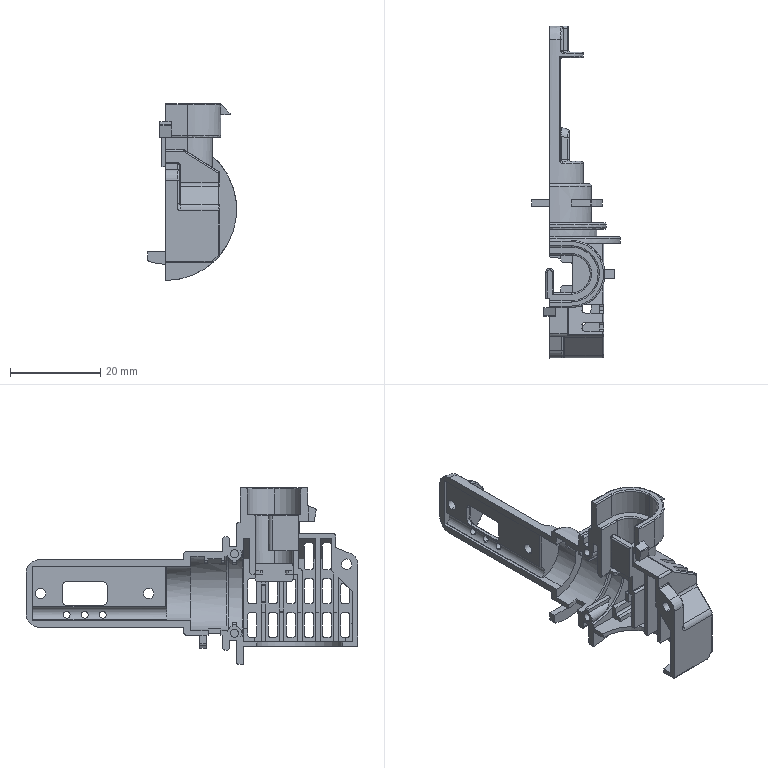Part | SolidWorks | features ICE 12, MoveFace 5, BaseBody 1, Chamfer 1 | 1 solid | 542 faces | box 19.75 x 73.802 x 39.25 mm | volume 4726 mm3 | plane 243 | cylinder 209 | spline 81 | cone 6 | torus 3 | commonest cylinder face diameters 1 x79 0.6 x70 2 x7 1.5 x6 2.3 x6 3.6 x6